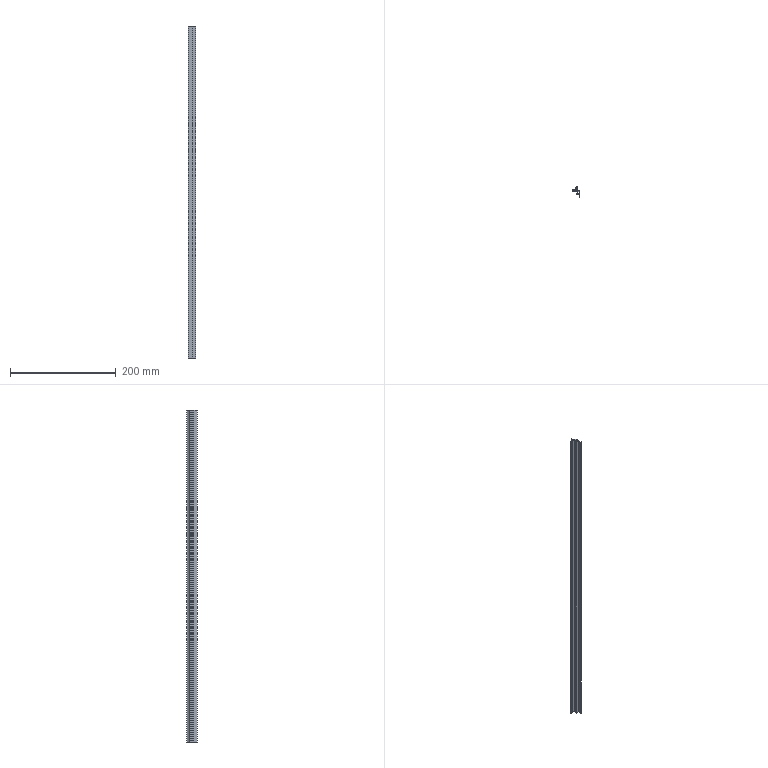Part | SolidWorks | features BaseBody 1, ICE 1, MoveFace 1 | 1 solid | 27 faces | box 14 x 20.3 x 627 mm | volume 31924 mm3 | plane 20 | cylinder 7 | commonest cylinder face diameters 0.387 x2 0.8 x2 0.4 x1 20 x1 22 x1
STEP:
#1=CARTESIAN_POINT('',(-5.304,-0.625,200.));
#2=VERTEX_POINT('',#1);
#3=CARTESIAN_POINT('',(-5.449,-0.8125,200.));
#4=VERTEX_POINT('',#3);
#5=CARTESIAN_POINT('',(-5.255,-0.8125,200.));
#6=DIRECTION('',(0.,0.,1.));
#7=DIRECTION('',(-1.,0.,0.));
#8=AXIS2_PLACEMENT_3D('',#5,#6,#7);
#9=CIRCLE('',#8,0.1937);
#10=EDGE_CURVE('',#2,#4,#9,.T.);
#11=ORIENTED_EDGE('',*,*,#10,.T.);
#12=CARTESIAN_POINT('',(-5.449,-0.8125,-427.));
#13=VERTEX_POINT('',#12);
#14=CARTESIAN_POINT('',(-5.449,-0.8125,230.));
#15=DIRECTION('',(0.,0.,-1.));
#16=VECTOR('',#15,1000.);
#17=LINE('',#14,#16);
#18=EDGE_CURVE('',#4,#13,#17,.T.);
#19=ORIENTED_EDGE('',*,*,#18,.T.);
#20=CARTESIAN_POINT('',(-5.304,-0.625,-427.));
#21=VERTEX_POINT('',#20);
#22=CARTESIAN_POINT('',(-5.255,-0.8125,-427.));
#23=DIRECTION('',(0.,0.,-1.));
#24=DIRECTION('',(1.,0.,0.));
#25=AXIS2_PLACEMENT_3D('',#22,#23,#24);
#26=CIRCLE('',#25,0.1937);
#27=EDGE_CURVE('',#13,#21,#26,.T.);
#28=ORIENTED_EDGE('',*,*,#27,.T.);
#29=CARTESIAN_POINT('',(-5.304,-0.625,230.));
#30=DIRECTION('',(0.,0.,-1.));
#31=VECTOR('',#30,1000.);
#32=LINE('',#29,#31);
#33=EDGE_CURVE('',#2,#21,#32,.T.);
#34=ORIENTED_EDGE('',*,*,#33,.F.);
#35=EDGE_LOOP('',(#11,#19,#28,#34));
#36=FACE_OUTER_BOUND('',#35,.T.);
#37=CARTESIAN_POINT('',(-5.255,-0.8125,230.));
#38=DIRECTION('',(0.,0.,-1.));
#39=DIRECTION('',(-1.,0.,0.));
#40=AXIS2_PLACEMENT_3D('',#37,#38,#39);
#41=CYLINDRICAL_SURFACE('',#40,0.1937);
#42=ADVANCED_FACE('',(#36),#41,.F.);
#43=CARTESIAN_POINT('',(5.,-1.,-427.));
#44=VERTEX_POINT('',#43);
#45=CARTESIAN_POINT('',(5.,-14.3,-427.));
#46=VERTEX_POINT('',#45);
#47=CARTESIAN_POINT('',(5.,29.623,-427.));
#48=DIRECTION('',(0.,-1.,0.));
#49=VECTOR('',#48,1000.);
#50=LINE('',#47,#49);
#51=EDGE_CURVE('',#44,#46,#50,.T.);
#52=ORIENTED_EDGE('',*,*,#51,.F.);
#53=CARTESIAN_POINT('',(5.,-1.,200.));
#54=VERTEX_POINT('',#53);
#55=CARTESIAN_POINT('',(5.,-1.,230.));
#56=DIRECTION('',(0.,0.,-1.));
#57=VECTOR('',#56,1000.);
#58=LINE('',#55,#57);
#59=EDGE_CURVE('',#54,#44,#58,.T.);
#60=ORIENTED_EDGE('',*,*,#59,.F.);
#61=CARTESIAN_POINT('',(5.,-14.3,200.));
#62=VERTEX_POINT('',#61);
#63=CARTESIAN_POINT('',(5.,-14.3,200.));
#64=DIRECTION('',(0.,1.,0.));
#65=VECTOR('',#64,1000.);
#66=LINE('',#63,#65);
#67=EDGE_CURVE('',#62,#54,#66,.T.);
#68=ORIENTED_EDGE('',*,*,#67,.F.);
#69=CARTESIAN_POINT('',(5.,-14.3,230.));
#70=DIRECTION('',(0.,0.,1.));
#71=VECTOR('',#70,1000.);
#72=LINE('',#69,#71);
#73=EDGE_CURVE('',#46,#62,#72,.T.);
#74=ORIENTED_EDGE('',*,*,#73,.F.);
#75=EDGE_LOOP('',(#52,#60,#68,#74));
#76=FACE_OUTER_BOUND('',#75,.T.);
#77=CARTESIAN_POINT('',(5.,-14.3,230.));
#78=DIRECTION('',(-1.,0.,0.));
#79=DIRECTION('',(0.,0.,1.));
#80=AXIS2_PLACEMENT_3D('',#77,#78,#79);
#81=PLANE('',#80);
#82=ADVANCED_FACE('',(#76),#81,.F.);
#83=CARTESIAN_POINT('',(-9.,-2.,-427.));
#84=VERTEX_POINT('',#83);
#85=CARTESIAN_POINT('',(-9.,-2.,200.));
#86=VERTEX_POINT('',#85);
#87=CARTESIAN_POINT('',(-9.,-2.,230.));
#88=DIRECTION('',(0.,0.,1.));
#89=VECTOR('',#88,1000.);
#90=LINE('',#87,#89);
#91=EDGE_CURVE('',#84,#86,#90,.T.);
#92=ORIENTED_EDGE('',*,*,#91,.F.);
#93=CARTESIAN_POINT('',(0.9,-2.,-427.));
#94=VERTEX_POINT('',#93);
#95=CARTESIAN_POINT('',(5.,-2.,-427.));
#96=DIRECTION('',(-1.,0.,0.));
#97=VECTOR('',#96,1000.);
#98=LINE('',#95,#97);
#99=EDGE_CURVE('',#94,#84,#98,.T.);
#100=ORIENTED_EDGE('',*,*,#99,.F.);
#101=CARTESIAN_POINT('',(0.9,-2.,200.));
#102=VERTEX_POINT('',#101);
#103=CARTESIAN_POINT('',(0.9,-2.,230.));
#104=DIRECTION('',(0.,0.,-1.));
#105=VECTOR('',#104,1000.);
#106=LINE('',#103,#105);
#107=EDGE_CURVE('',#102,#94,#106,.T.);
#108=ORIENTED_EDGE('',*,*,#107,.F.);
#109=CARTESIAN_POINT('',(5.,-2.,200.));
#110=DIRECTION('',(1.,0.,0.));
#111=VECTOR('',#110,1000.);
#112=LINE('',#109,#111);
#113=EDGE_CURVE('',#86,#102,#112,.T.);
#114=ORIENTED_EDGE('',*,*,#113,.F.);
#115=EDGE_LOOP('',(#92,#100,#108,#114));
#116=FACE_OUTER_BOUND('',#115,.T.);
#117=CARTESIAN_POINT('',(-9.,-2.,230.));
#118=DIRECTION('',(0.,1.,0.));
#119=DIRECTION('',(0.,0.,1.));
#120=AXIS2_PLACEMENT_3D('',#117,#118,#119);
#121=PLANE('',#120);
#122=ADVANCED_FACE('',(#116),#121,.F.);
#123=CARTESIAN_POINT('',(4.,-6.,200.));
#124=VERTEX_POINT('',#123);
#125=CARTESIAN_POINT('',(4.,-3.,200.));
#126=VERTEX_POINT('',#125);
#127=CARTESIAN_POINT('',(4.,29.623,200.));
#128=DIRECTION('',(0.,1.,0.));
#129=VECTOR('',#128,1000.);
#130=LINE('',#127,#129);
#131=EDGE_CURVE('',#124,#126,#130,.T.);
#132=ORIENTED_EDGE('',*,*,#131,.F.);
#133=CARTESIAN_POINT('',(1.,-6.,200.));
#134=VERTEX_POINT('',#133);
#135=CARTESIAN_POINT('',(5.,-6.,200.));
#136=DIRECTION('',(1.,0.,0.));
#137=VECTOR('',#136,1000.);
#138=LINE('',#135,#137);
#139=EDGE_CURVE('',#134,#124,#138,.T.);
#140=ORIENTED_EDGE('',*,*,#139,.F.);
#141=CARTESIAN_POINT('',(1.,-6.7,200.));
#142=VERTEX_POINT('',#141);
#143=CARTESIAN_POINT('',(1.,-6.,200.));
#144=DIRECTION('',(0.,-1.,0.));
#145=VECTOR('',#144,1000.);
#146=LINE('',#143,#145);
#147=EDGE_CURVE('',#134,#142,#146,.T.);
#148=ORIENTED_EDGE('',*,*,#147,.T.);
#149=CARTESIAN_POINT('',(-1.7,-6.7,200.));
#150=VERTEX_POINT('',#149);
#151=CARTESIAN_POINT('',(5.,-6.7,200.));
#152=DIRECTION('',(1.,0.,0.));
#153=VECTOR('',#152,1000.);
#154=LINE('',#151,#153);
#155=EDGE_CURVE('',#150,#142,#154,.T.);
#156=ORIENTED_EDGE('',*,*,#155,.F.);
#157=CARTESIAN_POINT('',(-1.7,-7.7,200.));
#158=VERTEX_POINT('',#157);
#159=CARTESIAN_POINT('',(-1.7,-6.7,200.));
#160=DIRECTION('',(0.,-1.,0.));
#161=VECTOR('',#160,1000.);
#162=LINE('',#159,#161);
#163=EDGE_CURVE('',#150,#158,#162,.T.);
#164=ORIENTED_EDGE('',*,*,#163,.T.);
#165=CARTESIAN_POINT('',(4.,-7.7,200.));
#166=VERTEX_POINT('',#165);
#167=CARTESIAN_POINT('',(5.,-7.7,200.));
#168=DIRECTION('',(-1.,0.,0.));
#169=VECTOR('',#168,1000.);
#170=LINE('',#167,#169);
#171=EDGE_CURVE('',#166,#158,#170,.T.);
#172=ORIENTED_EDGE('',*,*,#171,.F.);
#173=CARTESIAN_POINT('',(4.,-14.3,200.));
#174=VERTEX_POINT('',#173);
#175=CARTESIAN_POINT('',(4.,29.623,200.));
#176=DIRECTION('',(0.,1.,0.));
#177=VECTOR('',#176,1000.);
#178=LINE('',#175,#177);
#179=EDGE_CURVE('',#174,#166,#178,.T.);
#180=ORIENTED_EDGE('',*,*,#179,.F.);
#181=CARTESIAN_POINT('',(5.,-14.3,200.));
#182=DIRECTION('',(-1.,0.,0.));
#183=VECTOR('',#182,1000.);
#184=LINE('',#181,#183);
#185=EDGE_CURVE('',#62,#174,#184,.T.);
#186=ORIENTED_EDGE('',*,*,#185,.F.);
#187=ORIENTED_EDGE('',*,*,#67,.T.);
#188=CARTESIAN_POINT('',(-5.207,-1.,200.));
#189=VERTEX_POINT('',#188);
#190=CARTESIAN_POINT('',(5.,-1.,200.));
#191=DIRECTION('',(1.,0.,0.));
#192=VECTOR('',#191,1000.);
#193=LINE('',#190,#192);
#194=EDGE_CURVE('',#189,#54,#193,.T.);
#195=ORIENTED_EDGE('',*,*,#194,.F.);
#196=CARTESIAN_POINT('',(-5.255,-0.8125,200.));
#197=DIRECTION('',(0.,0.,1.));
#198=DIRECTION('',(-1.,0.,0.));
#199=AXIS2_PLACEMENT_3D('',#196,#197,#198);
#200=CIRCLE('',#199,0.1937);
#201=EDGE_CURVE('',#4,#189,#200,.T.);
#202=ORIENTED_EDGE('',*,*,#201,.F.);
#203=ORIENTED_EDGE('',*,*,#10,.F.);
#204=CARTESIAN_POINT('',(-1.368,3.063,200.));
#205=VERTEX_POINT('',#204);
#206=CARTESIAN_POINT('',(-10.628,9.,200.));
#207=DIRECTION('',(0.,0.,1.));
#208=DIRECTION('',(-1.,0.,0.));
#209=AXIS2_PLACEMENT_3D('',#206,#207,#208);
#210=CIRCLE('',#209,11.);
#211=EDGE_CURVE('',#2,#205,#210,.T.);
#212=ORIENTED_EDGE('',*,*,#211,.T.);
#213=CARTESIAN_POINT('',(-1.,2.955,200.));
#214=VERTEX_POINT('',#213);
#215=CARTESIAN_POINT('',(-1.2,2.955,200.));
#216=DIRECTION('',(0.,0.,1.));
#217=DIRECTION('',(-1.,0.,0.));
#218=AXIS2_PLACEMENT_3D('',#215,#216,#217);
#219=CIRCLE('',#218,0.2);
#220=EDGE_CURVE('',#214,#205,#219,.T.);
#221=ORIENTED_EDGE('',*,*,#220,.F.);
#222=CARTESIAN_POINT('',(-1.,1.5,200.));
#223=VERTEX_POINT('',#222);
#224=CARTESIAN_POINT('',(-1.,2.955,200.));
#225=DIRECTION('',(0.,1.,0.));
#226=VECTOR('',#225,1000.);
#227=LINE('',#224,#226);
#228=EDGE_CURVE('',#223,#214,#227,.T.);
#229=ORIENTED_EDGE('',*,*,#228,.F.);
#230=CARTESIAN_POINT('',(0.,1.5,200.));
#231=VERTEX_POINT('',#230);
#232=CARTESIAN_POINT('',(-1.,1.5,200.));
#233=DIRECTION('',(-1.,0.,0.));
#234=VECTOR('',#233,1000.);
#235=LINE('',#232,#234);
#236=EDGE_CURVE('',#231,#223,#235,.T.);
#237=ORIENTED_EDGE('',*,*,#236,.F.);
#238=CARTESIAN_POINT('',(0.,6.,200.));
#239=VERTEX_POINT('',#238);
#240=CARTESIAN_POINT('',(0.,1.5,200.));
#241=DIRECTION('',(0.,-1.,0.));
#242=VECTOR('',#241,1000.);
#243=LINE('',#240,#242);
#244=EDGE_CURVE('',#239,#231,#243,.T.);
#245=ORIENTED_EDGE('',*,*,#244,.F.);
#246=CARTESIAN_POINT('',(-0.8,6.,200.));
#247=VERTEX_POINT('',#246);
#248=CARTESIAN_POINT('',(0.,6.,200.));
#249=DIRECTION('',(1.,0.,0.));
#250=VECTOR('',#249,1000.);
#251=LINE('',#248,#250);
#252=EDGE_CURVE('',#247,#239,#251,.T.);
#253=ORIENTED_EDGE('',*,*,#252,.F.);
#254=CARTESIAN_POINT('',(-1.178,5.731,200.));
#255=VERTEX_POINT('',#254);
#256=CARTESIAN_POINT('',(-0.8,5.6,200.));
#257=DIRECTION('',(0.,0.,1.));
#258=DIRECTION('',(-1.,0.,0.));
#259=AXIS2_PLACEMENT_3D('',#256,#257,#258);
#260=CIRCLE('',#259,0.4);
#261=EDGE_CURVE('',#247,#255,#260,.T.);
#262=ORIENTED_EDGE('',*,*,#261,.T.);
#263=CARTESIAN_POINT('',(-8.678,-0.8077,200.));
#264=VERTEX_POINT('',#263);
#265=CARTESIAN_POINT('',(-10.628,9.,200.));
#266=DIRECTION('',(0.,0.,1.));
#267=DIRECTION('',(-1.,0.,0.));
#268=AXIS2_PLACEMENT_3D('',#265,#266,#267);
#269=CIRCLE('',#268,10.);
#270=EDGE_CURVE('',#264,#255,#269,.T.);
#271=ORIENTED_EDGE('',*,*,#270,.F.);
#272=CARTESIAN_POINT('',(-9.,-1.2,200.));
#273=VERTEX_POINT('',#272);
#274=CARTESIAN_POINT('',(-8.6,-1.2,200.));
#275=DIRECTION('',(0.,0.,1.));
#276=DIRECTION('',(-1.,0.,0.));
#277=AXIS2_PLACEMENT_3D('',#274,#275,#276);
#278=CIRCLE('',#277,0.4);
#279=EDGE_CURVE('',#264,#273,#278,.T.);
#280=ORIENTED_EDGE('',*,*,#279,.T.);
#281=CARTESIAN_POINT('',(-9.,8.,200.));
#282=DIRECTION('',(0.,-1.,0.));
#283=VECTOR('',#282,1000.);
#284=LINE('',#281,#283);
#285=EDGE_CURVE('',#273,#86,#284,.T.);
#286=ORIENTED_EDGE('',*,*,#285,.T.);
#287=ORIENTED_EDGE('',*,*,#113,.T.);
#288=CARTESIAN_POINT('',(0.9,-3.,200.));
#289=VERTEX_POINT('',#288);
#290=CARTESIAN_POINT('',(0.9,29.623,200.));
#291=DIRECTION('',(0.,1.,0.));
#292=VECTOR('',#291,1000.);
#293=LINE('',#290,#292);
#294=EDGE_CURVE('',#289,#102,#293,.T.);
#295=ORIENTED_EDGE('',*,*,#294,.F.);
#296=CARTESIAN_POINT('',(5.,-3.,200.));
#297=DIRECTION('',(-1.,0.,0.));
#298=VECTOR('',#297,1000.);
#299=LINE('',#296,#298);
#300=EDGE_CURVE('',#126,#289,#299,.T.);
#301=ORIENTED_EDGE('',*,*,#300,.F.);
#302=EDGE_LOOP('',(#132,#140,#148,#156,#164,#172,#180,#186,#187,#195,#202,#203,#212,#221,#229,#237,#245,#253,#262,#271,#280,#286,#287,#295,#301));
#303=FACE_OUTER_BOUND('',#302,.T.);
#304=CARTESIAN_POINT('',(5.,29.623,200.));
#305=DIRECTION('',(0.,0.,-1.));
#306=DIRECTION('',(-1.,0.,0.));
#307=AXIS2_PLACEMENT_3D('',#304,#305,#306);
#308=PLANE('',#307);
#309=ADVANCED_FACE('',(#303),#308,.F.);
#310=ORIENTED_EDGE('',*,*,#185,.T.);
#311=CARTESIAN_POINT('',(4.,-14.3,-427.));
#312=VERTEX_POINT('',#311);
#313=CARTESIAN_POINT('',(4.,-14.3,230.));
#314=DIRECTION('',(0.,0.,1.));
#315=VECTOR('',#314,1000.);
#316=LINE('',#313,#315);
#317=EDGE_CURVE('',#312,#174,#316,.T.);
#318=ORIENTED_EDGE('',*,*,#317,.F.);
#319=CARTESIAN_POINT('',(5.,-14.3,-427.));
#320=DIRECTION('',(-1.,0.,0.));
#321=VECTOR('',#320,1000.);
#322=LINE('',#319,#321);
#323=EDGE_CURVE('',#46,#312,#322,.T.);
#324=ORIENTED_EDGE('',*,*,#323,.F.);
#325=ORIENTED_EDGE('',*,*,#73,.T.);
#326=EDGE_LOOP('',(#310,#318,#324,#325));
#327=FACE_OUTER_BOUND('',#326,.T.);
#328=CARTESIAN_POINT('',(4.,-14.3,230.));
#329=DIRECTION('',(0.,1.,0.));
#330=DIRECTION('',(0.,0.,1.));
#331=AXIS2_PLACEMENT_3D('',#328,#329,#330);
#332=PLANE('',#331);
#333=ADVANCED_FACE('',(#327),#332,.F.);
#334=ORIENTED_EDGE('',*,*,#51,.T.);
#335=ORIENTED_EDGE('',*,*,#323,.T.);
#336=CARTESIAN_POINT('',(4.,-7.7,-427.));
#337=VERTEX_POINT('',#336);
#338=CARTESIAN_POINT('',(4.,-7.7,-427.));
#339=DIRECTION('',(0.,-1.,0.));
#340=VECTOR('',#339,1000.);
#341=LINE('',#338,#340);
#342=EDGE_CURVE('',#337,#312,#341,.T.);
#343=ORIENTED_EDGE('',*,*,#342,.F.);
#344=CARTESIAN_POINT('',(-1.7,-7.7,-427.));
#345=VERTEX_POINT('',#344);
#346=CARTESIAN_POINT('',(-1.7,-7.7,-427.));
#347=DIRECTION('',(1.,0.,0.));
#348=VECTOR('',#347,1000.);
#349=LINE('',#346,#348);
#350=EDGE_CURVE('',#345,#337,#349,.T.);
#351=ORIENTED_EDGE('',*,*,#350,.F.);
#352=CARTESIAN_POINT('',(-1.7,-6.7,-427.));
#353=VERTEX_POINT('',#352);
#354=CARTESIAN_POINT('',(-1.7,29.623,-427.));
#355=DIRECTION('',(0.,1.,0.));
#356=VECTOR('',#355,1000.);
#357=LINE('',#354,#356);
#358=EDGE_CURVE('',#345,#353,#357,.T.);
#359=ORIENTED_EDGE('',*,*,#358,.T.);
#360=CARTESIAN_POINT('',(1.,-6.7,-427.));
#361=VERTEX_POINT('',#360);
#362=CARTESIAN_POINT('',(1.,-6.7,-427.));
#363=DIRECTION('',(-1.,0.,0.));
#364=VECTOR('',#363,1000.);
#365=LINE('',#362,#364);
#366=EDGE_CURVE('',#361,#353,#365,.T.);
#367=ORIENTED_EDGE('',*,*,#366,.F.);
#368=CARTESIAN_POINT('',(1.,-6.,-427.));
#369=VERTEX_POINT('',#368);
#370=CARTESIAN_POINT('',(1.,29.623,-427.));
#371=DIRECTION('',(0.,1.,0.));
#372=VECTOR('',#371,1000.);
#373=LINE('',#370,#372);
#374=EDGE_CURVE('',#361,#369,#373,.T.);
#375=ORIENTED_EDGE('',*,*,#374,.T.);
#376=CARTESIAN_POINT('',(4.,-6.,-427.));
#377=VERTEX_POINT('',#376);
#378=CARTESIAN_POINT('',(4.,-6.,-427.));
#379=DIRECTION('',(-1.,0.,0.));
#380=VECTOR('',#379,1000.);
#381=LINE('',#378,#380);
#382=EDGE_CURVE('',#377,#369,#381,.T.);
#383=ORIENTED_EDGE('',*,*,#382,.F.);
#384=CARTESIAN_POINT('',(4.,-3.,-427.));
#385=VERTEX_POINT('',#384);
#386=CARTESIAN_POINT('',(4.,-3.,-427.));
#387=DIRECTION('',(0.,-1.,0.));
#388=VECTOR('',#387,1000.);
#389=LINE('',#386,#388);
#390=EDGE_CURVE('',#385,#377,#389,.T.);
#391=ORIENTED_EDGE('',*,*,#390,.F.);
#392=CARTESIAN_POINT('',(0.9,-3.,-427.));
#393=VERTEX_POINT('',#392);
#394=CARTESIAN_POINT('',(0.9,-3.,-427.));
#395=DIRECTION('',(1.,0.,0.));
#396=VECTOR('',#395,1000.);
#397=LINE('',#394,#396);
#398=EDGE_CURVE('',#393,#385,#397,.T.);
#399=ORIENTED_EDGE('',*,*,#398,.F.);
#400=CARTESIAN_POINT('',(0.9,-2.,-427.));
#401=DIRECTION('',(0.,-1.,0.));
#402=VECTOR('',#401,1000.);
#403=LINE('',#400,#402);
#404=EDGE_CURVE('',#94,#393,#403,.T.);
#405=ORIENTED_EDGE('',*,*,#404,.F.);
#406=ORIENTED_EDGE('',*,*,#99,.T.);
#407=CARTESIAN_POINT('',(-9.,-1.2,-427.));
#408=VERTEX_POINT('',#407);
#409=CARTESIAN_POINT('',(-9.,-1.2,-427.));
#410=DIRECTION('',(0.,-1.,0.));
#411=VECTOR('',#410,1000.);
#412=LINE('',#409,#411);
#413=EDGE_CURVE('',#408,#84,#412,.T.);
#414=ORIENTED_EDGE('',*,*,#413,.F.);
#415=CARTESIAN_POINT('',(-8.678,-0.8077,-427.));
#416=VERTEX_POINT('',#415);
#417=CARTESIAN_POINT('',(-8.6,-1.2,-427.));
#418=DIRECTION('',(0.,0.,-1.));
#419=DIRECTION('',(1.,0.,0.));
#420=AXIS2_PLACEMENT_3D('',#417,#418,#419);
#421=CIRCLE('',#420,0.4);
#422=EDGE_CURVE('',#408,#416,#421,.T.);
#423=ORIENTED_EDGE('',*,*,#422,.T.);
#424=CARTESIAN_POINT('',(-1.178,5.731,-427.));
#425=VERTEX_POINT('',#424);
#426=CARTESIAN_POINT('',(-10.628,9.,-427.));
#427=DIRECTION('',(0.,0.,-1.));
#428=DIRECTION('',(1.,0.,0.));
#429=AXIS2_PLACEMENT_3D('',#426,#427,#428);
#430=CIRCLE('',#429,10.);
#431=EDGE_CURVE('',#425,#416,#430,.T.);
#432=ORIENTED_EDGE('',*,*,#431,.F.);
#433=CARTESIAN_POINT('',(-0.8,6.,-427.));
#434=VERTEX_POINT('',#433);
#435=CARTESIAN_POINT('',(-0.8,5.6,-427.));
#436=DIRECTION('',(0.,0.,-1.));
#437=DIRECTION('',(1.,0.,0.));
#438=AXIS2_PLACEMENT_3D('',#435,#436,#437);
#439=CIRCLE('',#438,0.4);
#440=EDGE_CURVE('',#425,#434,#439,.T.);
#441=ORIENTED_EDGE('',*,*,#440,.T.);
#442=CARTESIAN_POINT('',(0.,6.,-427.));
#443=VERTEX_POINT('',#442);
#444=CARTESIAN_POINT('',(0.,6.,-427.));
#445=DIRECTION('',(-1.,0.,0.));
#446=VECTOR('',#445,1000.);
#447=LINE('',#444,#446);
#448=EDGE_CURVE('',#443,#434,#447,.T.);
#449=ORIENTED_EDGE('',*,*,#448,.F.);
#450=CARTESIAN_POINT('',(0.,1.5,-427.));
#451=VERTEX_POINT('',#450);
#452=CARTESIAN_POINT('',(0.,1.5,-427.));
#453=DIRECTION('',(0.,1.,0.));
#454=VECTOR('',#453,1000.);
#455=LINE('',#452,#454);
#456=EDGE_CURVE('',#451,#443,#455,.T.);
#457=ORIENTED_EDGE('',*,*,#456,.F.);
#458=CARTESIAN_POINT('',(-1.,1.5,-427.));
#459=VERTEX_POINT('',#458);
#460=CARTESIAN_POINT('',(-1.,1.5,-427.));
#461=DIRECTION('',(1.,0.,0.));
#462=VECTOR('',#461,1000.);
#463=LINE('',#460,#462);
#464=EDGE_CURVE('',#459,#451,#463,.T.);
#465=ORIENTED_EDGE('',*,*,#464,.F.);
#466=CARTESIAN_POINT('',(-1.,2.955,-427.));
#467=VERTEX_POINT('',#466);
#468=CARTESIAN_POINT('',(-1.,2.955,-427.));
#469=DIRECTION('',(0.,-1.,0.));
#470=VECTOR('',#469,1000.);
#471=LINE('',#468,#470);
#472=EDGE_CURVE('',#467,#459,#471,.T.);
#473=ORIENTED_EDGE('',*,*,#472,.F.);
#474=CARTESIAN_POINT('',(-1.368,3.063,-427.));
#475=VERTEX_POINT('',#474);
#476=CARTESIAN_POINT('',(-1.2,2.955,-427.));
#477=DIRECTION('',(0.,0.,-1.));
#478=DIRECTION('',(1.,0.,0.));
#479=AXIS2_PLACEMENT_3D('',#476,#477,#478);
#480=CIRCLE('',#479,0.2);
#481=EDGE_CURVE('',#475,#467,#480,.T.);
#482=ORIENTED_EDGE('',*,*,#481,.F.);
#483=CARTESIAN_POINT('',(-10.628,9.,-427.));
#484=DIRECTION('',(0.,0.,-1.));
#485=DIRECTION('',(1.,0.,0.));
#486=AXIS2_PLACEMENT_3D('',#483,#484,#485);
#487=CIRCLE('',#486,11.);
#488=EDGE_CURVE('',#475,#21,#487,.T.);
#489=ORIENTED_EDGE('',*,*,#488,.T.);
#490=ORIENTED_EDGE('',*,*,#27,.F.);
#491=CARTESIAN_POINT('',(-5.207,-1.,-427.));
#492=VERTEX_POINT('',#491);
#493=CARTESIAN_POINT('',(-5.255,-0.8125,-427.));
#494=DIRECTION('',(0.,0.,-1.));
#495=DIRECTION('',(1.,0.,0.));
#496=AXIS2_PLACEMENT_3D('',#493,#494,#495);
#497=CIRCLE('',#496,0.1937);
#498=EDGE_CURVE('',#492,#13,#497,.T.);
#499=ORIENTED_EDGE('',*,*,#498,.F.);
#500=CARTESIAN_POINT('',(5.,-1.,-427.));
#501=DIRECTION('',(-1.,0.,0.));
#502=VECTOR('',#501,1000.);
#503=LINE('',#500,#502);
#504=EDGE_CURVE('',#44,#492,#503,.T.);
#505=ORIENTED_EDGE('',*,*,#504,.F.);
#506=EDGE_LOOP('',(#334,#335,#343,#351,#359,#367,#375,#383,#391,#399,#405,#406,#414,#423,#432,#441,#449,#457,#465,#473,#482,#489,#490,#499,#505));
#507=FACE_OUTER_BOUND('',#506,.T.);
#508=CARTESIAN_POINT('',(5.,29.623,-427.));
#509=DIRECTION('',(0.,0.,1.));
#510=DIRECTION('',(1.,0.,0.));
#511=AXIS2_PLACEMENT_3D('',#508,#509,#510);
#512=PLANE('',#511);
#513=ADVANCED_FACE('',(#507),#512,.F.);
#514=ORIENTED_EDGE('',*,*,#59,.T.);
#515=ORIENTED_EDGE('',*,*,#504,.T.);
#516=CARTESIAN_POINT('',(-5.207,-1.,230.));
#517=DIRECTION('',(0.,0.,-1.));
#518=VECTOR('',#517,1000.);
#519=LINE('',#516,#518);
#520=EDGE_CURVE('',#189,#492,#519,.T.);
#521=ORIENTED_EDGE('',*,*,#520,.F.);
#522=ORIENTED_EDGE('',*,*,#194,.T.);
#523=EDGE_LOOP('',(#514,#515,#521,#522));
#524=FACE_OUTER_BOUND('',#523,.T.);
#525=CARTESIAN_POINT('',(5.,-1.,230.));
#526=DIRECTION('',(0.,-1.,0.));
#527=DIRECTION('',(0.,0.,-1.));
#528=AXIS2_PLACEMENT_3D('',#525,#526,#527);
#529=PLANE('',#528);
#530=ADVANCED_FACE('',(#524),#529,.F.);
#531=CARTESIAN_POINT('',(-9.,-1.2,230.));
#532=DIRECTION('',(0.,0.,1.));
#533=VECTOR('',#532,1000.);
#534=LINE('',#531,#533);
#535=EDGE_CURVE('',#408,#273,#534,.T.);
#536=ORIENTED_EDGE('',*,*,#535,.F.);
#537=ORIENTED_EDGE('',*,*,#413,.T.);
#538=ORIENTED_EDGE('',*,*,#91,.T.);
#539=ORIENTED_EDGE('',*,*,#285,.F.);
#540=EDGE_LOOP('',(#536,#537,#538,#539));
#541=FACE_OUTER_BOUND('',#540,.T.);
#542=CARTESIAN_POINT('',(-9.,-1.2,230.));
#543=DIRECTION('',(1.,0.,0.));
#544=DIRECTION('',(0.,0.,-1.));
#545=AXIS2_PLACEMENT_3D('',#542,#543,#544);
#546=PLANE('',#545);
#547=ADVANCED_FACE('',(#541),#546,.F.);
#548=ORIENTED_EDGE('',*,*,#294,.T.);
#549=ORIENTED_EDGE('',*,*,#107,.T.);
#550=ORIENTED_EDGE('',*,*,#404,.T.);
#551=CARTESIAN_POINT('',(0.9,-3.,230.));
#552=DIRECTION('',(0.,0.,-1.));
#553=VECTOR('',#552,1000.);
#554=LINE('',#551,#553);
#555=EDGE_CURVE('',#289,#393,#554,.T.);
#556=ORIENTED_EDGE('',*,*,#555,.F.);
#557=EDGE_LOOP('',(#548,#549,#550,#556));
#558=FACE_OUTER_BOUND('',#557,.T.);
#559=CARTESIAN_POINT('',(0.9,-2.,230.));
#560=DIRECTION('',(1.,0.,0.));
#561=DIRECTION('',(0.,0.,-1.));
#562=AXIS2_PLACEMENT_3D('',#559,#560,#561);
#563=PLANE('',#562);
#564=ADVANCED_FACE('',(#558),#563,.F.);
#565=ORIENTED_EDGE('',*,*,#300,.T.);
#566=ORIENTED_EDGE('',*,*,#555,.T.);
#567=ORIENTED_EDGE('',*,*,#398,.T.);
#568=CARTESIAN_POINT('',(4.,-3.,230.));
#569=DIRECTION('',(0.,0.,-1.));
#570=VECTOR('',#569,1000.);
#571=LINE('',#568,#570);
#572=EDGE_CURVE('',#126,#385,#571,.T.);
#573=ORIENTED_EDGE('',*,*,#572,.F.);
#574=EDGE_LOOP('',(#565,#566,#567,#573));
#575=FACE_OUTER_BOUND('',#574,.T.);
#576=CARTESIAN_POINT('',(0.9,-3.,230.));
#577=DIRECTION('',(0.,1.,0.));
#578=DIRECTION('',(0.,0.,1.));
#579=AXIS2_PLACEMENT_3D('',#576,#577,#578);
#580=PLANE('',#579);
#581=ADVANCED_FACE('',(#575),#580,.F.);
#582=ORIENTED_EDGE('',*,*,#131,.T.);
#583=ORIENTED_EDGE('',*,*,#572,.T.);
#584=ORIENTED_EDGE('',*,*,#390,.T.);
#585=CARTESIAN_POINT('',(4.,-6.,230.));
#586=DIRECTION('',(0.,0.,-1.));
#587=VECTOR('',#586,1000.);
#588=LINE('',#585,#587);
#589=EDGE_CURVE('',#124,#377,#588,.T.);
#590=ORIENTED_EDGE('',*,*,#589,.F.);
#591=EDGE_LOOP('',(#582,#583,#584,#590));
#592=FACE_OUTER_BOUND('',#591,.T.);
#593=CARTESIAN_POINT('',(4.,-3.,230.));
#594=DIRECTION('',(1.,0.,0.));
#595=DIRECTION('',(0.,0.,-1.));
#596=AXIS2_PLACEMENT_3D('',#593,#594,#595);
#597=PLANE('',#596);
#598=ADVANCED_FACE('',(#592),#597,.F.);
#599=ORIENTED_EDGE('',*,*,#139,.T.);
#600=ORIENTED_EDGE('',*,*,#589,.T.);
#601=ORIENTED_EDGE('',*,*,#382,.T.);
#602=CARTESIAN_POINT('',(1.,-6.,230.));
#603=DIRECTION('',(0.,0.,-1.));
#604=VECTOR('',#603,1000.);
#605=LINE('',#602,#604);
#606=EDGE_CURVE('',#134,#369,#605,.T.);
#607=ORIENTED_EDGE('',*,*,#606,.F.);
#608=EDGE_LOOP('',(#599,#600,#601,#607));
#609=FACE_OUTER_BOUND('',#608,.T.);
#610=CARTESIAN_POINT('',(4.,-6.,230.));
#611=DIRECTION('',(0.,-1.,0.));
#612=DIRECTION('',(0.,0.,-1.));
#613=AXIS2_PLACEMENT_3D('',#610,#611,#612);
#614=PLANE('',#613);
#615=ADVANCED_FACE('',(#609),#614,.F.);
#616=ORIENTED_EDGE('',*,*,#155,.T.);
#617=CARTESIAN_POINT('',(1.,-6.7,230.));
#618=DIRECTION('',(0.,0.,1.));
#619=VECTOR('',#618,1000.);
#620=LINE('',#617,#619);
#621=EDGE_CURVE('',#361,#142,#620,.T.);
#622=ORIENTED_EDGE('',*,*,#621,.F.);
#623=ORIENTED_EDGE('',*,*,#366,.T.);
#624=CARTESIAN_POINT('',(-1.7,-6.7,230.));
#625=DIRECTION('',(0.,0.,-1.));
#626=VECTOR('',#625,1000.);
#627=LINE('',#624,#626);
#628=EDGE_CURVE('',#150,#353,#627,.T.);
#629=ORIENTED_EDGE('',*,*,#628,.F.);
#630=EDGE_LOOP('',(#616,#622,#623,#629));
#631=FACE_OUTER_BOUND('',#630,.T.);
#632=CARTESIAN_POINT('',(1.,-6.7,230.));
#633=DIRECTION('',(0.,-1.,0.));
#634=DIRECTION('',(0.,0.,-1.));
#635=AXIS2_PLACEMENT_3D('',#632,#633,#634);
#636=PLANE('',#635);
#637=ADVANCED_FACE('',(#631),#636,.F.);
#638=ORIENTED_EDGE('',*,*,#171,.T.);
#639=CARTESIAN_POINT('',(-1.7,-7.7,230.));
#640=DIRECTION('',(0.,0.,1.));
#641=VECTOR('',#640,1000.);
#642=LINE('',#639,#641);
#643=EDGE_CURVE('',#345,#158,#642,.T.);
#644=ORIENTED_EDGE('',*,*,#643,.F.);
#645=ORIENTED_EDGE('',*,*,#350,.T.);
#646=CARTESIAN_POINT('',(4.,-7.7,230.));
#647=DIRECTION('',(0.,0.,-1.));
#648=VECTOR('',#647,1000.);
#649=LINE('',#646,#648);
#650=EDGE_CURVE('',#166,#337,#649,.T.);
#651=ORIENTED_EDGE('',*,*,#650,.F.);
#652=EDGE_LOOP('',(#638,#644,#645,#651));
#653=FACE_OUTER_BOUND('',#652,.T.);
#654=CARTESIAN_POINT('',(-1.7,-7.7,230.));
#655=DIRECTION('',(0.,1.,0.));
#656=DIRECTION('',(0.,0.,1.));
#657=AXIS2_PLACEMENT_3D('',#654,#655,#656);
#658=PLANE('',#657);
#659=ADVANCED_FACE('',(#653),#658,.F.);
#660=ORIENTED_EDGE('',*,*,#179,.T.);
#661=ORIENTED_EDGE('',*,*,#650,.T.);
#662=ORIENTED_EDGE('',*,*,#342,.T.);
#663=ORIENTED_EDGE('',*,*,#317,.T.);
#664=EDGE_LOOP('',(#660,#661,#662,#663));
#665=FACE_OUTER_BOUND('',#664,.T.);
#666=CARTESIAN_POINT('',(4.,-7.7,230.));
#667=DIRECTION('',(1.,0.,0.));
#668=DIRECTION('',(0.,0.,-1.));
#669=AXIS2_PLACEMENT_3D('',#666,#667,#668);
#670=PLANE('',#669);
#671=ADVANCED_FACE('',(#665),#670,.F.);
#672=ORIENTED_EDGE('',*,*,#18,.F.);
#673=ORIENTED_EDGE('',*,*,#201,.T.);
#674=ORIENTED_EDGE('',*,*,#520,.T.);
#675=ORIENTED_EDGE('',*,*,#498,.T.);
#676=EDGE_LOOP('',(#672,#673,#674,#675));
#677=FACE_OUTER_BOUND('',#676,.T.);
#678=CARTESIAN_POINT('',(-5.255,-0.8125,230.));
#679=DIRECTION('',(0.,0.,-1.));
#680=DIRECTION('',(-1.,0.,0.));
#681=AXIS2_PLACEMENT_3D('',#678,#679,#680);
#682=CYLINDRICAL_SURFACE('',#681,0.1937);
#683=ADVANCED_FACE('',(#677),#682,.F.);
#684=CARTESIAN_POINT('',(-1.,2.955,230.));
#685=DIRECTION('',(0.,0.,1.));
#686=VECTOR('',#685,1000.);
#687=LINE('',#684,#686);
#688=EDGE_CURVE('',#467,#214,#687,.T.);
#689=ORIENTED_EDGE('',*,*,#688,.F.);
#690=ORIENTED_EDGE('',*,*,#472,.T.);
#691=CARTESIAN_POINT('',(-1.,1.5,230.));
#692=DIRECTION('',(0.,0.,-1.));
#693=VECTOR('',#692,1000.);
#694=LINE('',#691,#693);
#695=EDGE_CURVE('',#223,#459,#694,.T.);
#696=ORIENTED_EDGE('',*,*,#695,.F.);
#697=ORIENTED_EDGE('',*,*,#228,.T.);
#698=EDGE_LOOP('',(#689,#690,#696,#697));
#699=FACE_OUTER_BOUND('',#698,.T.);
#700=CARTESIAN_POINT('',(-1.,2.955,230.));
#701=DIRECTION('',(1.,0.,0.));
#702=DIRECTION('',(0.,0.,-1.));
#703=AXIS2_PLACEMENT_3D('',#700,#701,#702);
#704=PLANE('',#703);
#705=ADVANCED_FACE('',(#699),#704,.F.);
#706=ORIENTED_EDGE('',*,*,#488,.F.);
#707=CARTESIAN_POINT('',(-1.368,3.063,230.));
#708=DIRECTION('',(0.,0.,1.));
#709=VECTOR('',#708,1000.);
#710=LINE('',#707,#709);
#711=EDGE_CURVE('',#475,#205,#710,.T.);
#712=ORIENTED_EDGE('',*,*,#711,.T.);
#713=ORIENTED_EDGE('',*,*,#211,.F.);
#714=ORIENTED_EDGE('',*,*,#33,.T.);
#715=EDGE_LOOP('',(#706,#712,#713,#714));
#716=FACE_OUTER_BOUND('',#715,.T.);
#717=CARTESIAN_POINT('',(-10.628,9.,230.));
#718=DIRECTION('',(0.,0.,-1.));
#719=DIRECTION('',(-1.,0.,0.));
#720=AXIS2_PLACEMENT_3D('',#717,#718,#719);
#721=CYLINDRICAL_SURFACE('',#720,11.);
#722=ADVANCED_FACE('',(#716),#721,.T.);
#723=CARTESIAN_POINT('',(-1.178,5.731,230.));
#724=DIRECTION('',(0.,0.,1.));
#725=VECTOR('',#724,1000.);
#726=LINE('',#723,#725);
#727=EDGE_CURVE('',#425,#255,#726,.T.);
#728=ORIENTED_EDGE('',*,*,#727,.F.);
#729=ORIENTED_EDGE('',*,*,#431,.T.);
#730=CARTESIAN_POINT('',(-8.678,-0.8077,230.));
#731=DIRECTION('',(0.,0.,-1.));
#732=VECTOR('',#731,1000.);
#733=LINE('',#730,#732);
#734=EDGE_CURVE('',#264,#416,#733,.T.);
#735=ORIENTED_EDGE('',*,*,#734,.F.);
#736=ORIENTED_EDGE('',*,*,#270,.T.);
#737=EDGE_LOOP('',(#728,#729,#735,#736));
#738=FACE_OUTER_BOUND('',#737,.T.);
#739=CARTESIAN_POINT('',(-10.628,9.,230.));
#740=DIRECTION('',(0.,0.,-1.));
#741=DIRECTION('',(-1.,0.,0.));
#742=AXIS2_PLACEMENT_3D('',#739,#740,#741);
#743=CYLINDRICAL_SURFACE('',#742,10.);
#744=ADVANCED_FACE('',(#738),#743,.F.);
#745=CARTESIAN_POINT('',(0.,1.5,230.));
#746=DIRECTION('',(0.,0.,1.));
#747=VECTOR('',#746,1000.);
#748=LINE('',#745,#747);
#749=EDGE_CURVE('',#451,#231,#748,.T.);
#750=ORIENTED_EDGE('',*,*,#749,.F.);
#751=ORIENTED_EDGE('',*,*,#456,.T.);
#752=CARTESIAN_POINT('',(0.,6.,230.));
#753=DIRECTION('',(0.,0.,-1.));
#754=VECTOR('',#753,1000.);
#755=LINE('',#752,#754);
#756=EDGE_CURVE('',#239,#443,#755,.T.);
#757=ORIENTED_EDGE('',*,*,#756,.F.);
#758=ORIENTED_EDGE('',*,*,#244,.T.);
#759=EDGE_LOOP('',(#750,#751,#757,#758));
#760=FACE_OUTER_BOUND('',#759,.T.);
#761=CARTESIAN_POINT('',(0.,1.5,230.));
#762=DIRECTION('',(-1.,0.,0.));
#763=DIRECTION('',(0.,0.,1.));
#764=AXIS2_PLACEMENT_3D('',#761,#762,#763);
#765=PLANE('',#764);
#766=ADVANCED_FACE('',(#760),#765,.F.);
#767=ORIENTED_EDGE('',*,*,#422,.F.);
#768=ORIENTED_EDGE('',*,*,#535,.T.);
#769=ORIENTED_EDGE('',*,*,#279,.F.);
#770=ORIENTED_EDGE('',*,*,#734,.T.);
#771=EDGE_LOOP('',(#767,#768,#769,#770));
#772=FACE_OUTER_BOUND('',#771,.T.);
#773=CARTESIAN_POINT('',(-8.6,-1.2,230.));
#774=DIRECTION('',(0.,0.,-1.));
#775=DIRECTION('',(-1.,0.,0.));
#776=AXIS2_PLACEMENT_3D('',#773,#774,#775);
#777=CYLINDRICAL_SURFACE('',#776,0.4);
#778=ADVANCED_FACE('',(#772),#777,.T.);
#779=ORIENTED_EDGE('',*,*,#147,.F.);
#780=ORIENTED_EDGE('',*,*,#606,.T.);
#781=ORIENTED_EDGE('',*,*,#374,.F.);
#782=ORIENTED_EDGE('',*,*,#621,.T.);
#783=EDGE_LOOP('',(#779,#780,#781,#782));
#784=FACE_OUTER_BOUND('',#783,.T.);
#785=CARTESIAN_POINT('',(1.,-6.,230.));
#786=DIRECTION('',(1.,0.,0.));
#787=DIRECTION('',(0.,0.,-1.));
#788=AXIS2_PLACEMENT_3D('',#785,#786,#787);
#789=PLANE('',#788);
#790=ADVANCED_FACE('',(#784),#789,.F.);
#791=ORIENTED_EDGE('',*,*,#163,.F.);
#792=ORIENTED_EDGE('',*,*,#628,.T.);
#793=ORIENTED_EDGE('',*,*,#358,.F.);
#794=ORIENTED_EDGE('',*,*,#643,.T.);
#795=EDGE_LOOP('',(#791,#792,#793,#794));
#796=FACE_OUTER_BOUND('',#795,.T.);
#797=CARTESIAN_POINT('',(-1.7,-6.7,230.));
#798=DIRECTION('',(1.,0.,0.));
#799=DIRECTION('',(0.,0.,-1.));
#800=AXIS2_PLACEMENT_3D('',#797,#798,#799);
#801=PLANE('',#800);
#802=ADVANCED_FACE('',(#796),#801,.F.);
#803=ORIENTED_EDGE('',*,*,#711,.F.);
#804=ORIENTED_EDGE('',*,*,#481,.T.);
#805=ORIENTED_EDGE('',*,*,#688,.T.);
#806=ORIENTED_EDGE('',*,*,#220,.T.);
#807=EDGE_LOOP('',(#803,#804,#805,#806));
#808=FACE_OUTER_BOUND('',#807,.T.);
#809=CARTESIAN_POINT('',(-1.2,2.955,230.));
#810=DIRECTION('',(0.,0.,-1.));
#811=DIRECTION('',(-1.,0.,0.));
#812=AXIS2_PLACEMENT_3D('',#809,#810,#811);
#813=CYLINDRICAL_SURFACE('',#812,0.2);
#814=ADVANCED_FACE('',(#808),#813,.F.);
#815=ORIENTED_EDGE('',*,*,#695,.T.);
#816=ORIENTED_EDGE('',*,*,#464,.T.);
#817=ORIENTED_EDGE('',*,*,#749,.T.);
#818=ORIENTED_EDGE('',*,*,#236,.T.);
#819=EDGE_LOOP('',(#815,#816,#817,#818));
#820=FACE_OUTER_BOUND('',#819,.T.);
#821=CARTESIAN_POINT('',(-1.,1.5,230.));
#822=DIRECTION('',(0.,1.,0.));
#823=DIRECTION('',(0.,0.,1.));
#824=AXIS2_PLACEMENT_3D('',#821,#822,#823);
#825=PLANE('',#824);
#826=ADVANCED_FACE('',(#820),#825,.F.);
#827=ORIENTED_EDGE('',*,*,#440,.F.);
#828=ORIENTED_EDGE('',*,*,#727,.T.);
#829=ORIENTED_EDGE('',*,*,#261,.F.);
#830=CARTESIAN_POINT('',(-0.8,6.,230.));
#831=DIRECTION('',(0.,0.,-1.));
#832=VECTOR('',#831,1000.);
#833=LINE('',#830,#832);
#834=EDGE_CURVE('',#247,#434,#833,.T.);
#835=ORIENTED_EDGE('',*,*,#834,.T.);
#836=EDGE_LOOP('',(#827,#828,#829,#835));
#837=FACE_OUTER_BOUND('',#836,.T.);
#838=CARTESIAN_POINT('',(-0.8,5.6,230.));
#839=DIRECTION('',(0.,0.,-1.));
#840=DIRECTION('',(-1.,0.,0.));
#841=AXIS2_PLACEMENT_3D('',#838,#839,#840);
#842=CYLINDRICAL_SURFACE('',#841,0.4);
#843=ADVANCED_FACE('',(#837),#842,.T.);
#844=ORIENTED_EDGE('',*,*,#756,.T.);
#845=ORIENTED_EDGE('',*,*,#448,.T.);
#846=ORIENTED_EDGE('',*,*,#834,.F.);
#847=ORIENTED_EDGE('',*,*,#252,.T.);
#848=EDGE_LOOP('',(#844,#845,#846,#847));
#849=FACE_OUTER_BOUND('',#848,.T.);
#850=CARTESIAN_POINT('',(0.,6.,230.));
#851=DIRECTION('',(0.,-1.,0.));
#852=DIRECTION('',(0.,0.,-1.));
#853=AXIS2_PLACEMENT_3D('',#850,#851,#852);
#854=PLANE('',#853);
#855=ADVANCED_FACE('',(#849),#854,.F.);
#856=CLOSED_SHELL('',(#42,#82,#122,#309,#333,#513,#530,#547,#564,#581,#598,#615,#637,#659,#671,#683,#705,#722,#744,#766,#778,#790,#802,#814,#826,#843,#855));
#857=MANIFOLD_SOLID_BREP('',#856);
#858=CARTESIAN_POINT('',(0.,0.,0.));
#859=DIRECTION('',(0.,0.,1.));
#860=DIRECTION('',(1.,0.,0.));
#861=AXIS2_PLACEMENT_3D('',#858,#859,#860);
#862=(LENGTH_UNIT()NAMED_UNIT(*)SI_UNIT(.MILLI.,.METRE.));
#863=UNCERTAINTY_MEASURE_WITH_UNIT(LENGTH_MEASURE(0.00001),#862,'','');
#864=(NAMED_UNIT(*)PLANE_ANGLE_UNIT()SI_UNIT($,.RADIAN.));
#865=(NAMED_UNIT(*)SI_UNIT($,.STERADIAN.)SOLID_ANGLE_UNIT());
#866=(GEOMETRIC_REPRESENTATION_CONTEXT(3)GLOBAL_UNCERTAINTY_ASSIGNED_CONTEXT((#863))GLOBAL_UNIT_ASSIGNED_CONTEXT((#862,#864,#865))REPRESENTATION_CONTEXT('',''));
#867=ADVANCED_BREP_SHAPE_REPRESENTATION('',(#857,#861),#866);